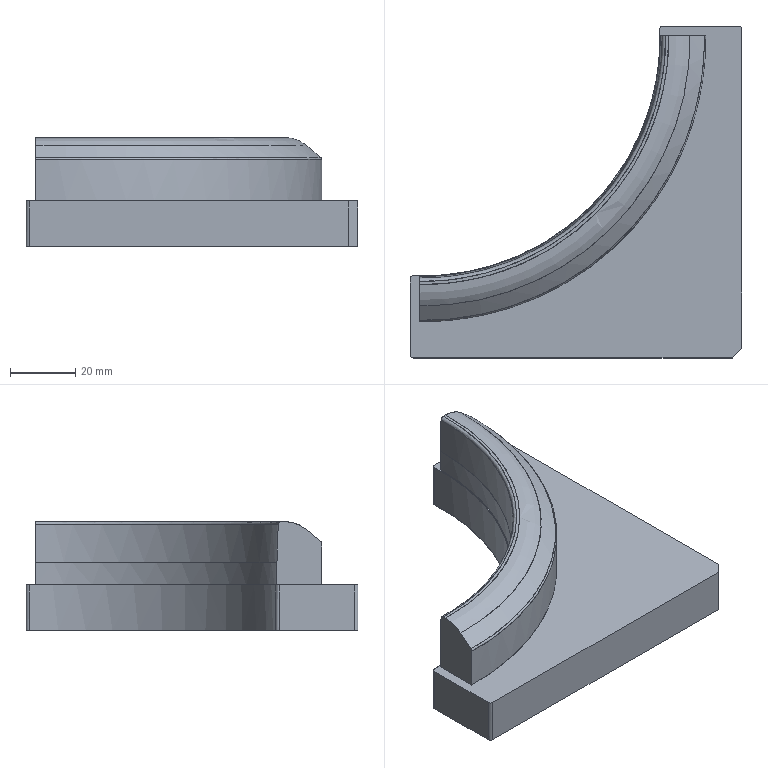NC program | PowerMill | posted with a generic post | part box 102 x 102 x 33.478 mm
Lines 27281 to 27988 of 205885:
N27378 M6
N27379 S18000 M03
N27380 G00 G90 X0.0 Y0.0
N27381 G43 Z10.798 H7
N27382
N27383 G05 P10000 R8
N27384 X16.2265 Y-15.1208
N27385 Z-7.8611
N27386 G01 Z-9.0611 F1200.0
N27387 X16.2193 Y-15.128 Z-9.0578 F2000.0
N27388 X16.1176 Y-15.2297 Z-9.0126
N27389 X16.0433 Y-15.304 Z-8.9841
N27390 X15.9799 Y-15.3673 Z-8.9661
N27391 X15.9402 Y-15.4071 Z-8.9595
N27392 X15.9003 Y-15.447 Z-8.9553
N27393 X15.8603 Y-15.4869 Z-8.9522
N27394 X15.7961 Y-15.5511 Z-8.9488
N27395 X15.7542 Y-15.593 Z-8.9473
N27396 X15.7142 Y-15.6331 Z-8.9464
N27397 X15.6741 Y-15.6732 Z-8.9466
N27398 X15.5794 Y-15.7678 Z-8.952
N27399 X15.4849 Y-15.8624 Z-8.9611
N27400 X15.39 Y-15.9572 Z-8.972
N27401 X15.2955 Y-16.0517 Z-8.9829
N27402 X15.2717 Y-16.0756 Z-8.9874
N27403 X15.2451 Y-16.1021 Z-8.9994
N27404 X15.2228 Y-16.1245 Z-9.0128
N27405 X15.1913 Y-16.1559 Z-9.0307
N27406 X15.1262 Y-16.2211 Z-9.0616
N27407 X13.2708 Y-17.9916 Z-9.0896
N27408 Z-9.0776
N27409 X13.2828 Y-17.9797 Z-9.0118
N27410 X13.2897 Y-17.9727 Z-8.9971
N27411 X13.3018 Y-17.9606 Z-8.9768
N27412 X13.3197 Y-17.9427 Z-8.9513
N27413 X13.3315 Y-17.931 Z-8.9371
N27414 X13.3421 Y-17.9203 Z-8.9277
N27415 X13.4059 Y-17.8566 Z-8.8821
N27416 X13.4779 Y-17.7845 Z-8.839
N27417 X13.5611 Y-17.7013 Z-8.7974
N27418 X13.6507 Y-17.6117 Z-8.7595
N27419 X13.7504 Y-17.512 Z-8.725
N27420 X13.8798 Y-17.3826 Z-8.687
N27421 X13.9702 Y-17.2922 Z-8.6636
N27422 X14.0609 Y-17.2015 Z-8.6432
N27423 X14.1517 Y-17.1107 Z-8.6243
N27424 X14.2427 Y-17.0197 Z-8.6067
N27425 X14.3339 Y-16.9286 Z-8.5905
N27426 X14.4252 Y-16.8372 Z-8.5767
N27427 X14.6885 Y-16.5739 Z-8.544
N27428 X14.9492 Y-16.3132 Z-8.5196
N27429 X15.2071 Y-16.0553 Z-8.5032
N27430 X15.4446 Y-15.8178 Z-8.4956
N27431 X15.7078 Y-15.5546 Z-8.4947
N27432 X15.9119 Y-15.3505 Z-8.4985
N27433 X16.1159 Y-15.1465 Z-8.5074
N27434 X16.3198 Y-14.9426 Z-8.5207
N27435 X16.5235 Y-14.7389 Z-8.5386
N27436 X16.7085 Y-14.5539 Z-8.5597
N27437 X16.8688 Y-14.3936 Z-8.5812
N27438 X17.0288 Y-14.2336 Z-8.6073
N27439 X17.1882 Y-14.0742 Z-8.6393
N27440 X17.2823 Y-13.9801 Z-8.6608
N27441 X17.4045 Y-13.8579 Z-8.6947
N27442 X17.4662 Y-13.7962 Z-8.7117
N27443 X17.506 Y-13.7564 Z-8.723
N27444 X17.5458 Y-13.7166 Z-8.7357
N27445 X17.5941 Y-13.6683 Z-8.7528
N27446 X17.6545 Y-13.6079 Z-8.7767
N27447 X17.7319 Y-13.5306 Z-8.812
N27448 X17.8001 Y-13.4623 Z-8.8488
N27449 X17.8538 Y-13.4086 Z-8.8833
N27450 X17.8968 Y-13.3656 Z-8.9163
N27451 X17.9314 Y-13.3311 Z-8.9484
N27452 X17.9522 Y-13.3102 Z-8.972
N27453 X17.9694 Y-13.293 Z-8.9998
N27454 X17.9824 Y-13.28 Z-9.0328
N27455 X17.9906 Y-13.2718 Z-9.0697
N27456 X17.9921 Y-13.2703 Z-9.0824
N27457 Z-9.0901
N27458 X18.8969 Y-12.2807 Z-9.0615
N27459 X18.8925 Y-12.285 Z-9.0442
N27460 X18.8789 Y-12.2987 Z-9.0058
N27461 X18.8582 Y-12.3194 Z-8.9636
N27462 X18.833 Y-12.3445 Z-8.9226
N27463 X18.8155 Y-12.3621 Z-8.8995
N27464 X18.7961 Y-12.3815 Z-8.8802
N27465 X18.7644 Y-12.4131 Z-8.8553
N27466 X18.7396 Y-12.438 Z-8.8355
N27467 X18.7035 Y-12.4741 Z-8.8076
N27468 X18.6614 Y-12.5162 Z-8.7799
N27469 X18.6104 Y-12.5671 Z-8.7504
N27470 X18.5454 Y-12.6322 Z-8.7168
N27471 X18.455 Y-12.7226 Z-8.6752
N27472 X18.3771 Y-12.8004 Z-8.6427
N27473 X18.3178 Y-12.8597 Z-8.6197
N27474 X18.2703 Y-12.9073 Z-8.6023
N27475 X18.2248 Y-12.9528 Z-8.5867
N27476 X18.1791 Y-12.9984 Z-8.5722
N27477 X18.103 Y-13.0746 Z-8.5503
N27478 X18.0267 Y-13.1509 Z-8.5296
N27479 X17.9503 Y-13.2273 Z-8.5095
N27480 X17.8697 Y-13.3078 Z-8.489
N27481 X17.7932 Y-13.3844 Z-8.4703
N27482 X17.7164 Y-13.4611 Z-8.4531
N27483 X17.6394 Y-13.5382 Z-8.4387
N27484 X17.4602 Y-13.7173 Z-8.4078
N27485 X17.2809 Y-13.8967 Z-8.3793
N27486 X17.1013 Y-14.0762 Z-8.3534
N27487 X16.9215 Y-14.256 Z-8.3317
N27488 X16.7123 Y-14.4653 Z-8.3122
N27489 X16.5029 Y-14.6746 Z-8.2962
N27490 X16.2935 Y-14.8841 Z-8.2832
N27491 X16.0839 Y-15.0936 Z-8.2736
N27492 X15.815 Y-15.3626 Z-8.2669
N27493 X15.4762 Y-15.7013 Z-8.2656
N27494 X15.1389 Y-16.0386 Z-8.2722
N27495 X14.936 Y-16.2416 Z-8.2803
N27496 X14.7331 Y-16.4445 Z-8.2919
N27497 X14.5303 Y-16.6473 Z-8.3068
N27498 X14.323 Y-16.8546 Z-8.3255
N27499 X14.1206 Y-17.057 Z-8.3479
N27500 X13.9185 Y-17.259 Z-8.3754
N27501 X13.7637 Y-17.4139 Z-8.4
N27502 X13.609 Y-17.5686 Z-8.4261
N27503 X13.4546 Y-17.723 Z-8.4556
N27504 X13.3008 Y-17.8768 Z-8.49
N27505 X13.1476 Y-18.0299 Z-8.53
N27506 X13.0554 Y-18.1221 Z-8.5567
N27507 X12.9635 Y-18.2141 Z-8.5851
N27508 X12.8718 Y-18.3057 Z-8.6155
N27509 X12.7807 Y-18.3968 Z-8.6487
N27510 X12.6905 Y-18.4871 Z-8.6862
N27511 X12.6162 Y-18.5613 Z-8.7234
N27512 X12.5356 Y-18.6419 Z-8.7718
N27513 X12.4413 Y-18.7362 Z-8.8361
N27514 X12.4063 Y-18.7713 Z-8.8615
N27515 X12.3731 Y-18.8044 Z-8.8915
N27516 X12.3433 Y-18.8342 Z-8.9278
N27517 X12.3174 Y-18.8602 Z-8.9699
N27518 X12.296 Y-18.8816 Z-9.0168
N27519 X12.2794 Y-18.8981 Z-9.0676
N27520 X11.518 Y-19.5747 Z-9.1132
N27521 Z-9.0836
N27522 X11.5206 Y-19.5721 Z-9.0598
N27523 X11.5261 Y-19.5666 Z-9.0337
N27524 X11.5372 Y-19.5555 Z-8.9982
N27525 X11.5536 Y-19.5391 Z-8.957
N27526 X11.5659 Y-19.5268 Z-8.9309
N27527 X11.5748 Y-19.5179 Z-8.9148
N27528 X11.5787 Y-19.514 Z-8.909
N27529 X11.6088 Y-19.4839 Z-8.8732
N27530 X11.6397 Y-19.453 Z-8.839
N27531 X11.6717 Y-19.421 Z-8.8073
N27532 X11.7052 Y-19.3875 Z-8.7786
N27533 X11.7477 Y-19.345 Z-8.7486
N27534 X11.784 Y-19.3087 Z-8.7262
N27535 X11.8206 Y-19.2721 Z-8.7046
N27536 X11.8571 Y-19.2356 Z-8.6828
N27537 X11.8933 Y-19.1994 Z-8.6604
N27538 X11.9298 Y-19.1629 Z-8.6399
N27539 X11.969 Y-19.1237 Z-8.6209
N27540 X12.0116 Y-19.0811 Z-8.6019
N27541 X12.0651 Y-19.0276 Z-8.5796
N27542 X12.1346 Y-18.9581 Z-8.5523
N27543 X12.2414 Y-18.8513 Z-8.5129
N27544 X12.3127 Y-18.78 Z-8.4879
N27545 X12.3676 Y-18.7251 Z-8.4695
N27546 X12.4116 Y-18.6811 Z-8.4552
N27547 X12.4522 Y-18.6405 Z-8.4426
N27548 X12.493 Y-18.5997 Z-8.4309
N27549 X12.6543 Y-18.4384 Z-8.3875
N27550 X12.816 Y-18.2767 Z-8.3473
N27551 X12.9784 Y-18.1143 Z-8.3128
N27552 X13.2181 Y-17.8746 Z-8.269
N27553 X13.5054 Y-17.5874 Z-8.2236
N27554 X13.738 Y-17.3547 Z-8.1922
N27555 X13.9711 Y-17.1217 Z-8.1664
N27556 X14.211 Y-16.8817 Z-8.1443
N27557 X14.4444 Y-16.6483 Z-8.1265
N27558 X14.678 Y-16.4147 Z-8.1123
N27559 X14.9116 Y-16.1811 Z-8.1017
N27560 X15.2722 Y-15.8205 Z-8.0917
N27561 X15.6329 Y-15.4598 Z-8.0897
N27562 X15.9569 Y-15.1358 Z-8.0946
N27563 X16.2808 Y-14.8119 Z-8.106
N27564 X16.6045 Y-14.4882 Z-8.1236
N27565 X16.928 Y-14.1647 Z-8.1479
N27566 X17.1899 Y-13.9028 Z-8.1731
N27567 X17.4514 Y-13.6413 Z-8.2043
N27568 X17.7125 Y-13.3802 Z-8.2424
N27569 X17.9731 Y-13.1196 Z-8.2864
N27570 X18.1574 Y-12.9353 Z-8.3214
N27571 X18.3526 Y-12.7401 Z-8.3658
N27572 X18.5738 Y-12.5189 Z-8.4236
N27573 X18.7134 Y-12.3793 Z-8.4638
N27574 X18.856 Y-12.2367 Z-8.512
N27575 X19.0069 Y-12.0858 Z-8.571
N27576 X19.0478 Y-12.0449 Z-8.5883
N27577 X19.1472 Y-11.9455 Z-8.634
N27578 X19.228 Y-11.8647 Z-8.6764
N27579 X19.295 Y-11.7978 Z-8.7162
N27580 X19.3511 Y-11.7416 Z-8.754
N27581 X19.3983 Y-11.6944 Z-8.7902
N27582 X19.4374 Y-11.6553 Z-8.825
N27583 X19.4707 Y-11.622 Z-8.8601
N27584 X19.4891 Y-11.6036 Z-8.8828
N27585 X19.5052 Y-11.5875 Z-8.9024
N27586 X19.5213 Y-11.5715 Z-8.9219
N27587 X19.5371 Y-11.5556 Z-8.9453
N27588 X19.5485 Y-11.5442 Z-8.9686
N27589 X19.558 Y-11.5347 Z-8.9937
N27590 X19.5651 Y-11.5276 Z-9.0157
N27591 X19.5699 Y-11.5228 Z-9.0391
N27592 X19.5739 Y-11.5188 Z-9.074
N27593 X19.5743 Y-11.5184 Z-9.0765
N27594 Z-9.1072
N27595 X20.1413 Y-10.8666 Z-9.0633
N27596 X20.1412 Y-10.8667 Z-9.0626
N27597 X20.1332 Y-10.8746 Z-9.0132
N27598 X20.1247 Y-10.8832 Z-8.9792
N27599 X20.114 Y-10.8938 Z-8.9541
N27600 X20.0833 Y-10.9246 Z-8.9013
N27601 X20.0491 Y-10.9587 Z-8.8526
N27602 X20.0109 Y-10.997 Z-8.8076
N27603 X19.9674 Y-11.0405 Z-8.7654
N27604 X19.9163 Y-11.0915 Z-8.7246
N27605 X19.8522 Y-11.1557 Z-8.6811
N27606 X19.7587 Y-11.2491 Z-8.6234
N27607 X19.6608 Y-11.3471 Z-8.5699
N27608 X19.5517 Y-11.4562 Z-8.5183
N27609 X19.4263 Y-11.5816 Z-8.467
N27610 X19.2723 Y-11.7355 Z-8.4112
N27611 X19.1728 Y-11.8351 Z-8.3774
N27612 X19.0434 Y-11.9644 Z-8.338
N27613 X18.9135 Y-12.0943 Z-8.3027
N27614 X18.7539 Y-12.2539 Z-8.263
N27615 X18.6233 Y-12.3846 Z-8.2328
N27616 X18.4925 Y-12.5154 Z-8.2042
N27617 X18.3542 Y-12.6536 Z-8.1768
N27618 X18.1829 Y-12.8249 Z-8.1467
N27619 X18.0113 Y-12.9965 Z-8.1194
N27620 X17.8396 Y-13.1683 Z-8.0942
N27621 X17.6677 Y-13.3402 Z-8.0709
N27622 X17.3611 Y-13.6467 Z-8.0352
N27623 X17.0339 Y-13.974 Z-8.0048
N27624 X16.6801 Y-14.3277 Z-7.9797
N27625 X16.2895 Y-14.7184 Z-7.9595
N27626 X16.1584 Y-14.8495 Z-7.9549
N27627 X16.0272 Y-14.9807 Z-7.9512
N27628 X15.896 Y-15.1118 Z-7.9479
N27629 X15.7649 Y-15.243 Z-7.9452
N27630 X15.4503 Y-15.5576 Z-7.9437
N27631 X15.0558 Y-15.9521 Z-7.9489
N27632 X14.6623 Y-16.3456 Z-7.9622
N27633 X14.2698 Y-16.738 Z-7.9833
N27634 X14.0453 Y-16.9625 Z-7.999
N27635 X13.821 Y-17.1869 Z-8.0181
N27636 X13.5967 Y-17.4111 Z-8.0406
N27637 X13.3727 Y-17.6351 Z-8.0664
N27638 X13.149 Y-17.8589 Z-8.0967
N27639 X12.8773 Y-18.1305 Z-8.1382
N27640 X12.6499 Y-18.358 Z-8.1774
N27641 X12.5531 Y-18.4547 Z-8.1965
N27642 X12.4565 Y-18.5514 Z-8.217
N27643 X12.36 Y-18.6479 Z-8.2384
N27644 X12.2635 Y-18.7443 Z-8.2606
N27645 X12.1672 Y-18.8406 Z-8.2837
N27646 X12.0711 Y-18.9368 Z-8.3081
N27647 X11.9752 Y-19.0326 Z-8.3346
N27648 X11.8798 Y-19.1281 Z-8.3644
N27649 X11.7783 Y-19.2296 Z-8.3969
N27650 X11.6769 Y-19.3309 Z-8.4306
N27651 X11.5668 Y-19.4411 Z-8.4709
N27652 X11.467 Y-19.5408 Z-8.5122
N27653 X11.3684 Y-19.6395 Z-8.5583
N27654 X11.2708 Y-19.737 Z-8.6089
N27655 X11.2003 Y-19.8076 Z-8.6489
N27656 X11.1276 Y-19.8803 Z-8.6962
N27657 X11.0661 Y-19.9418 Z-8.7432
N27658 X11.014 Y-19.9938 Z-8.7906
N27659 X10.9752 Y-20.0327 Z-8.8327
N27660 X10.937 Y-20.0708 Z-8.8832
N27661 X10.8932 Y-20.1146 Z-8.9506
N27662 X10.8824 Y-20.1255 Z-8.982
N27663 X10.871 Y-20.1369 Z-9.0303
N27664 X10.865 Y-20.1428 Z-9.0806
N27665 Z-9.0816
N27666 X10.2807 Y-20.6423 Z-9.0991
N27667 Z-9.0832
N27668 X10.2841 Y-20.6389 Z-9.043
N27669 X10.2908 Y-20.6322 Z-9.0038
N27670 X10.3022 Y-20.6208 Z-8.9661
N27671 X10.3174 Y-20.6056 Z-8.9318
N27672 X10.3352 Y-20.5878 Z-8.8991
N27673 X10.3678 Y-20.5552 Z-8.849
N27674 X10.407 Y-20.516 Z-8.8002
N27675 X10.4538 Y-20.4692 Z-8.7522
N27676 X10.5094 Y-20.4136 Z-8.7042
N27677 X10.5762 Y-20.3468 Z-8.6551
N27678 X10.6291 Y-20.2939 Z-8.6202
N27679 X10.7281 Y-20.1949 Z-8.5604
N27680 X10.8287 Y-20.0943 Z-8.5061
N27681 X10.9308 Y-19.9922 Z-8.4575
N27682 X11.0391 Y-19.8839 Z-8.412
N27683 X11.1433 Y-19.7797 Z-8.3725
N27684 X11.2478 Y-19.6752 Z-8.3353
N27685 X11.4165 Y-19.5065 Z-8.2809
N27686 X11.6143 Y-19.3087 Z-8.2247
N27687 X11.8201 Y-19.1029 Z-8.1719
N27688 X12.0406 Y-18.8824 Z-8.1225
N27689 X12.3038 Y-18.6192 Z-8.0707
N27690 X12.5005 Y-18.4225 Z-8.0354
N27691 X12.6977 Y-18.2253 Z-8.0047
N27692 X12.895 Y-18.028 Z-7.9773
N27693 X13.0925 Y-17.8305 Z-7.9518
N27694 X13.2902 Y-17.6328 Z-7.9283
N27695 X13.5397 Y-17.3833 Z-7.9032
N27696 X13.7895 Y-17.1335 Z-7.8815
N27697 X14.0394 Y-16.8836 Z-7.8632
N27698 X14.2894 Y-16.6336 Z-7.8486
N27699 X14.6538 Y-16.2692 Z-7.8326
N27700 X15.0183 Y-15.9047 Z-7.822
N27701 X15.3829 Y-15.5401 Z-7.8174
N27702 X15.7601 Y-15.1629 Z-7.8196
N27703 X16.1372 Y-14.7858 Z-7.8281
N27704 X16.5143 Y-14.4087 Z-7.8426
N27705 X16.8689 Y-14.0541 Z-7.8623
N27706 X17.2233 Y-13.6997 Z-7.8888
N27707 X17.5774 Y-13.3456 Z-7.9228
N27708 X17.9311 Y-12.9919 Z-7.9643
N27709 X18.1871 Y-12.7359 Z-7.9987
N27710 X18.4426 Y-12.4804 Z-8.039
N27711 X18.6976 Y-12.2254 Z-8.0855
N27712 X18.952 Y-11.971 Z-8.1378
N27713 X19.0809 Y-11.8421 Z-8.1666
N27714 X19.2094 Y-11.7136 Z-8.1981
N27715 X19.3376 Y-11.5854 Z-8.2322
N27716 X19.4822 Y-11.4408 Z-8.2739
N27717 X19.6095 Y-11.3135 Z-8.3135
N27718 X19.7363 Y-11.1867 Z-8.3565
N27719 X19.8623 Y-11.0607 Z-8.4042
N27720 X19.969 Y-10.954 Z-8.4488
N27721 X20.0876 Y-10.8354 Z-8.5035
N27722 X20.1634 Y-10.7596 Z-8.5427
N27723 X20.2476 Y-10.6754 Z-8.5903
N27724 X20.3319 Y-10.5911 Z-8.6437
N27725 X20.4041 Y-10.5189 Z-8.6966
N27726 X20.4709 Y-10.4521 Z-8.7535
N27727 X20.4973 Y-10.4257 Z-8.7785
N27728 X20.5195 Y-10.4035 Z-8.8028
N27729 X20.5441 Y-10.3789 Z-8.8347
N27730 X20.5757 Y-10.3473 Z-8.8825
N27731 X20.5998 Y-10.3232 Z-8.9256
N27732 X20.6156 Y-10.3074 Z-8.9603
N27733 X20.6262 Y-10.2968 Z-8.9908
N27734 X20.6368 Y-10.2862 Z-9.0304
N27735 X20.6415 Y-10.2815 Z-9.0635
N27736 X20.642 Y-10.281 Z-9.0766
N27737 Z-9.1018
N27738 X21.0919 Y-9.7462 Z-9.1082
N27739 Z-9.0725
N27740 Z-9.0709
N27741 X21.0896 Y-9.7486 Z-9.0535
N27742 X21.0871 Y-9.751 Z-9.0393
N27743 X21.0835 Y-9.7547 Z-9.0214
N27744 X21.0764 Y-9.7617 Z-8.993
N27745 X21.0663 Y-9.7718 Z-8.9581
N27746 X21.0592 Y-9.779 Z-8.9373
N27747 X21.0537 Y-9.7845 Z-8.9251
N27748 X21.0314 Y-9.8067 Z-8.8882
N27749 X21.0007 Y-9.8375 Z-8.8401
N27750 X20.9678 Y-9.8703 Z-8.795
N27751 X20.9324 Y-9.9057 Z-8.7541
N27752 X20.8947 Y-9.9434 Z-8.7175
N27753 X20.8556 Y-9.9826 Z-8.684
N27754 X20.8156 Y-10.0225 Z-8.6524
N27755 X20.7753 Y-10.0628 Z-8.622
N27756 X20.6917 Y-10.1464 Z-8.5649
N27757 X20.5988 Y-10.2394 Z-8.5099
N27758 X20.4936 Y-10.3445 Z-8.4558
N27759 X20.3904 Y-10.4477 Z-8.4075
N27760 X20.2744 Y-10.5638 Z-8.3567
N27761 X20.1573 Y-10.6808 Z-8.3107
N27762 X20.0393 Y-10.7988 Z-8.2694
N27763 X19.9208 Y-10.9173 Z-8.2312
N27764 X19.8021 Y-11.036 Z-8.1941
N27765 X19.6844 Y-11.1537 Z-8.1598
N27766 X19.5663 Y-11.2718 Z-8.1285
N27767 X19.448 Y-11.3901 Z-8.0989
N27768 X19.3295 Y-11.5086 Z-8.0707
N27769 X19.2109 Y-11.6273 Z-8.0438
N27770 X19.092 Y-11.7461 Z-8.0191
N27771 X18.8211 Y-12.0171 Z-7.9689
N27772 X18.5074 Y-12.3308 Z-7.9167
N27773 X18.2154 Y-12.6227 Z-7.8752
N27774 X17.8486 Y-12.9896 Z-7.8311
N27775 X17.4813 Y-13.3569 Z-7.794
N27776 X17.1137 Y-13.7245 Z-7.7639
N27777 X16.7246 Y-14.1135 Z-7.7393
N27778 X16.3354 Y-14.5027 Z-7.722
N27779 X15.9669 Y-14.8713 Z-7.7113
N27780 X15.5983 Y-15.2399 Z-7.7058
N27781 X15.2297 Y-15.6085 Z-7.7061
N27782 X14.7843 Y-16.0539 Z-7.7132
N27783 X14.3441 Y-16.494 Z-7.7281
N27784 X14.0453 Y-16.7928 Z-7.7433
N27785 X13.7466 Y-17.0915 Z-7.7625
N27786 X13.448 Y-17.3901 Z-7.7856
N27787 X13.2149 Y-17.6233 Z-7.8076
N27788 X12.9818 Y-17.8563 Z-7.8323
N27789 X12.7489 Y-18.0893 Z-7.8593
N27790 X12.5161 Y-18.322 Z-7.889
N27791 X12.3818 Y-18.4564 Z-7.9081
N27792 X12.2476 Y-18.5906 Z-7.9295
N27793 X12.1135 Y-18.7247 Z-7.9522
N27794 X11.9794 Y-18.8587 Z-7.9758
N27795 X11.8455 Y-18.9926 Z-8.0005
N27796 X11.7117 Y-19.1264 Z-8.0265
N27797 X11.5782 Y-19.2599 Z-8.055
N27798 X11.335 Y-19.5032 Z-8.1129
N27799 X11.1248 Y-19.7134 Z-8.168
N27800 X11.0262 Y-19.812 Z-8.1964
N27801 X10.9278 Y-19.9103 Z-8.2266
N27802 X10.8251 Y-20.013 Z-8.2603
N27803 X10.6985 Y-20.1397 Z-8.3051
N27804 X10.5457 Y-20.2925 Z-8.3645
N27805 X10.4274 Y-20.4107 Z-8.4157
N27806 X10.3305 Y-20.5076 Z-8.462
N27807 X10.2365 Y-20.6016 Z-8.512
N27808 X10.1667 Y-20.6714 Z-8.5536
N27809 X10.077 Y-20.7611 Z-8.6115
N27810 X10.0069 Y-20.8312 Z-8.6628
N27811 X9.9482 Y-20.89 Z-8.7131
N27812 X9.8976 Y-20.9405 Z-8.7643
N27813 X9.8535 Y-20.9847 Z-8.8178
N27814 X9.8304 Y-21.0078 Z-8.8495
N27815 X9.8091 Y-21.029 Z-8.8809
N27816 X9.7896 Y-21.0485 Z-8.9146
N27817 X9.7734 Y-21.0648 Z-8.9519
N27818 X9.7615 Y-21.0767 Z-8.9917
N27819 X9.7528 Y-21.0853 Z-9.0333
N27820 X9.746 Y-21.0922 Z-9.0756
N27821 Z-9.1074
N27822 X9.2611 Y-21.4922 Z-9.061
N27823 X9.2649 Y-21.4884 Z-9.0207
N27824 X9.2732 Y-21.4801 Z-8.9806
N27825 X9.2874 Y-21.4659 Z-8.9381
N27826 X9.3045 Y-21.4488 Z-8.8988
N27827 X9.3308 Y-21.4225 Z-8.8498
N27828 X9.3634 Y-21.3899 Z-8.8014
N27829 X9.4036 Y-21.3497 Z-8.7527
N27830 X9.4535 Y-21.2998 Z-8.7019
N27831 X9.5071 Y-21.2462 Z-8.654
N27832 X9.579 Y-21.1743 Z-8.5966
N27833 X9.6604 Y-21.0929 Z-8.5403
N27834 X9.7554 Y-20.9979 Z-8.483
N27835 X9.8729 Y-20.8804 Z-8.4196
N27836 X9.9927 Y-20.7606 Z-8.3616
N27837 X10.1299 Y-20.6234 Z-8.303
N27838 X10.2978 Y-20.4555 Z-8.2387
N27839 X10.4 Y-20.3533 Z-8.2018
N27840 X10.5028 Y-20.2505 Z-8.1685
N27841 X10.6059 Y-20.1474 Z-8.1373
N27842 X10.7092 Y-20.044 Z-8.1074
N27843 X10.8127 Y-19.9406 Z-8.0786
N27844 X10.9164 Y-19.8369 Z-8.0508
N27845 X11.0202 Y-19.7331 Z-8.0246
N27846 X11.1243 Y-19.629 Z-8.0007
N27847 X11.3783 Y-19.375 Z-7.946
N27848 X11.6328 Y-19.1204 Z-7.8966
N27849 X11.888 Y-18.8653 Z-7.8534
N27850 X12.1434 Y-18.6099 Z-7.8145
N27851 X12.3991 Y-18.3542 Z-7.779
N27852 X12.7088 Y-18.0445 Z-7.742
N27853 X13.0432 Y-17.7101 Z-7.7081
N27854 X13.3534 Y-17.3999 Z-7.6814
N27855 X13.6638 Y-17.0895 Z-7.6585
N27856 X14.077 Y-16.6763 Z-7.6344
N27857 X14.5028 Y-16.2505 Z-7.6171
N27858 X14.9549 Y-15.7984 Z-7.6066
N27859 X15.3833 Y-15.37 Z-7.6035
N27860 X15.8491 Y-14.9042 Z-7.6074
N27861 X16.3032 Y-14.4501 Z-7.6189
N27862 X16.7467 Y-14.0066 Z-7.6379
N27863 X17.1576 Y-13.5957 Z-7.663
N27864 X17.5842 Y-13.1691 Z-7.6969
N27865 X17.9183 Y-12.835 Z-7.7287
N27866 X18.252 Y-12.5013 Z-7.7661
N27867 X18.5853 Y-12.1679 Z-7.8106
N27868 X18.8431 Y-11.9102 Z-7.8498
N27869 X19.1006 Y-11.6527 Z-7.893
N27870 X19.3575 Y-11.3958 Z-7.9424
N27871 X19.5574 Y-11.1958 Z-7.9842
N27872 X19.7971 Y-10.9562 Z-8.04
N27873 X20.0184 Y-10.7349 Z-8.0988
N27874 X20.2254 Y-10.5279 Z-8.1612
N27875 X20.3961 Y-10.3572 Z-8.2187
N27876 X20.5023 Y-10.251 Z-8.2565
N27877 X20.6083 Y-10.145 Z-8.2957
N27878 X20.7134 Y-10.0399 Z-8.3389
N27879 X20.817 Y-9.9362 Z-8.3884
N27880 X20.9197 Y-9.8336 Z-8.4421
N27881 X20.9901 Y-9.7632 Z-8.4804
N27882 X21.0514 Y-9.7019 Z-8.5147
N27883 X21.1121 Y-9.6412 Z-8.5512
N27884 X21.1715 Y-9.5818 Z-8.5913
N27885 X21.2291 Y-9.5242 Z-8.6364
N27886 X21.2845 Y-9.4688 Z-8.6865
N27887 X21.338 Y-9.4153 Z-8.7407
N27888 X21.3672 Y-9.3861 Z-8.7721
N27889 X21.3799 Y-9.3734 Z-8.788
N27890 X21.3953 Y-9.358 Z-8.8097
N27891 X21.4191 Y-9.3342 Z-8.8459
N27892 X21.4356 Y-9.3177 Z-8.873
N27893 X21.4461 Y-9.3071 Z-8.8918
N27894 X21.4554 Y-9.2979 Z-8.9119
N27895 X21.4737 Y-9.2796 Z-8.9605
N27896 X21.4855 Y-9.2678 Z-9.0038
N27897 X21.4913 Y-9.262 Z-9.0423
N27898 X21.4922 Y-9.2611 Z-9.0632
N27899 X21.8673 Y-8.8012 Z-9.1297
N27900 Z-9.072
N27901 X21.8671 Y-8.8013 Z-9.0699
N27902 X21.8633 Y-8.8051 Z-9.016
N27903 X21.8572 Y-8.8112 Z-8.977
N27904 X21.8475 Y-8.8209 Z-8.9446
N27905 X21.8393 Y-8.8291 Z-8.9257
N27906 X21.8282 Y-8.8402 Z-8.9025
N27907 X21.8105 Y-8.858 Z-8.8674
N27908 X21.7911 Y-8.8773 Z-8.8318
N27909 X21.7778 Y-8.8907 Z-8.8095
N27910 X21.7667 Y-8.9017 Z-8.794
N27911 X21.7528 Y-8.9156 Z-8.778
N27912 X21.7027 Y-8.9657 Z-8.721
N27913 X21.6515 Y-9.017 Z-8.666
N27914 X21.5978 Y-9.0707 Z-8.6161
N27915 X21.5415 Y-9.127 Z-8.5725
N27916 X21.4836 Y-9.1848 Z-8.533
N27917 X21.4251 Y-9.2433 Z-8.4955
N27918 X21.3662 Y-9.3022 Z-8.4593
N27919 X21.247 Y-9.4214 Z-8.3919
N27920 X21.1183 Y-9.5501 Z-8.3275
N27921 X20.9777 Y-9.6907 Z-8.2653
N27922 X20.8211 Y-9.8473 Z-8.204
N27923 X20.6405 Y-10.028 Z-8.1408
N27924 X20.4152 Y-10.2532 Z-8.0693
N27925 X20.2912 Y-10.3772 Z-8.0329
N27926 X20.1362 Y-10.5322 Z-7.9924
N27927 X19.969 Y-10.6994 Z-7.9518
N27928 X19.8136 Y-10.8549 Z-7.9149
N27929 X19.6266 Y-11.0418 Z-7.8754
N27930 X19.4393 Y-11.2292 Z-7.8395
N27931 X19.2518 Y-11.4167 Z-7.8055
N27932 X18.947 Y-11.7215 Z-7.7553
N27933 X18.6416 Y-12.0268 Z-7.7122
N27934 X18.29 Y-12.3784 Z-7.6684
N27935 X17.9381 Y-12.7304 Z-7.6307
N27936 X17.5858 Y-13.0827 Z-7.5995
N27937 X17.2333 Y-13.4352 Z-7.5735
N27938 X16.7928 Y-13.8756 Z-7.5474
N27939 X16.3521 Y-14.3163 Z-7.5284
N27940 X15.8791 Y-14.7894 Z-7.5157
N27941 X15.3988 Y-15.2696 Z-7.5107
N27942 X14.9442 Y-15.7242 Z-7.5132
N27943 X14.4896 Y-16.1788 Z-7.5227
N27944 X14.0352 Y-16.6333 Z-7.5397
N27945 X13.5809 Y-17.0876 Z-7.5643
N27946 X13.196 Y-17.4725 Z-7.5904
N27947 X12.8349 Y-17.8336 Z-7.6207
N27948 X12.4741 Y-18.1943 Z-7.6577
N27949 X12.191 Y-18.4774 Z-7.6913
N27950 X11.9081 Y-18.7603 Z-7.7281
N27951 X11.7419 Y-18.9266 Z-7.7517
N27952 X11.5759 Y-19.0926 Z-7.7782
N27953 X11.41 Y-19.2584 Z-7.8068
N27954 X11.2443 Y-19.4242 Z-7.8368
N27955 X11.0787 Y-19.5898 Z-7.8682
N27956 X10.9133 Y-19.7551 Z-7.9019
N27957 X10.7483 Y-19.9201 Z-7.9394
N27958 X10.5566 Y-20.1119 Z-7.9866
N27959 X10.3653 Y-20.3032 Z-8.0373
N27960 X10.1746 Y-20.4938 Z-8.0926
N27961 X10.0934 Y-20.575 Z-8.1181
N27962 X10.0124 Y-20.6561 Z-8.1451
N27963 X9.925 Y-20.7434 Z-8.1758
N27964 X9.8204 Y-20.848 Z-8.2147
N27965 X9.6891 Y-20.9793 Z-8.2673
N27966 X9.5499 Y-21.1186 Z-8.3285
N27967 X9.4412 Y-21.2272 Z-8.381
N27968 X9.3517 Y-21.3168 Z-8.4286
N27969 X9.2751 Y-21.3934 Z-8.4733
N27970 X9.1998 Y-21.4687 Z-8.5223
N27971 X9.1443 Y-21.5242 Z-8.5628
N27972 X9.0662 Y-21.6022 Z-8.6228
N27973 X9.0088 Y-21.6596 Z-8.6725
N27974 X8.9623 Y-21.7061 Z-8.72
N27975 X8.9236 Y-21.7449 Z-8.768
N27976 X8.9019 Y-21.7665 Z-8.7981
N27977 X8.8784 Y-21.7901 Z-8.8322
N27978 X8.8572 Y-21.8113 Z-8.8661
N27979 X8.8386 Y-21.8299 Z-8.9019
N27980 X8.8231 Y-21.8453 Z-8.9425
N27981 X8.8128 Y-21.8556 Z-8.984
N27982 X8.806 Y-21.8624 Z-9.0268
N27983 X8.8012 Y-21.8672 Z-9.072
N27984 Y-21.8673 Z-9.1088
N27985 X8.3592 Y-22.2244 Z-9.0964
N27986 Z-9.0834
N27987 X8.3642 Y-22.2194 Z-9.0312
N27988 X8.3749 Y-22.2087 Z-8.9772
N27989 X8.3896 Y-22.194 Z-8.9296
N27990 X8.412 Y-22.1715 Z-8.8771
N27991 X8.4411 Y-22.1425 Z-8.8241
N27992 X8.4773 Y-22.1062 Z-8.7702
N27993 X8.5217 Y-22.0618 Z-8.7152
N27994 X8.5743 Y-22.0093 Z-8.6596
N27995 X8.6308 Y-21.9528 Z-8.6073
N27996 X8.7037 Y-21.8799 Z-8.5485
N27997 X8.7876 Y-21.796 Z-8.4895
N27998 X8.8878 Y-21.6958 Z-8.4271
N27999 X9.0151 Y-21.5685 Z-8.3555
N28000 X9.1492 Y-21.4343 Z-8.2883
N28001 X9.2951 Y-21.2884 Z-8.2233
N28002 X9.427 Y-21.1566 Z-8.1706
N28003 X9.5932 Y-20.9904 Z-8.1092
N28004 X9.7604 Y-20.8232 Z-8.0537
N28005 X9.9285 Y-20.6551 Z-8.0041
N28006 X10.1336 Y-20.45 Z-7.9471
N28007 X10.3392 Y-20.2444 Z-7.8945
N28008 X10.5456 Y-20.038 Z-7.848
N28009 X10.7523 Y-19.8313 Z-7.8046
N28010 X11.0157 Y-19.5679 Z-7.7541
N28011 X11.2888 Y-19.2948 Z-7.7083
N28012 X11.553 Y-19.0306 Z-7.6678
N28013 X11.8748 Y-18.7087 Z-7.6234
N28014 X12.1971 Y-18.3865 Z-7.5853
N28015 X12.5196 Y-18.064 Z-7.5521
N28016 X12.8423 Y-17.7413 Z-7.5229
N28017 X13.1651 Y-17.4184 Z-7.4978
N28018 X13.5764 Y-17.0072 Z-7.4721
N28019 X14.0541 Y-16.5295 Z-7.4498
N28020 X14.5319 Y-16.0517 Z-7.4349
N28021 X15.0098 Y-15.5738 Z-7.4271
N28022 X15.4544 Y-15.1291 Z-7.4262
N28023 X15.8991 Y-14.6845 Z-7.4316
N28024 X16.3437 Y-14.2399 Z-7.4432
N28025 X16.7882 Y-13.7954 Z-7.461
N28026 X17.2325 Y-13.3511 Z-7.4854
N28027 X17.5483 Y-13.0353 Z-7.5072
N28028 X17.8639 Y-12.7197 Z-7.5333
N28029 X18.3129 Y-12.2707 Z-7.5775
N28030 X18.6426 Y-11.941 Z-7.6151
N28031 X18.981 Y-11.6026 Z-7.6604
N28032 X19.333 Y-11.2506 Z-7.7142
N28033 X19.6299 Y-10.9537 Z-7.7655
N28034 X19.9085 Y-10.6751 Z-7.8205
N28035 X20.1804 Y-10.4031 Z-7.8802
N28036 X20.4202 Y-10.1634 Z-7.9395
N28037 X20.6156 Y-9.968 Z-7.9931
N28038 X20.8104 Y-9.7732 Z-8.051
N28039 X21.0042 Y-9.5794 Z-8.1149
N28040 X21.1805 Y-9.4031 Z-8.1785
N28041 X21.2285 Y-9.355 Z-8.1977
N28042 X21.2764 Y-9.3072 Z-8.2182
N28043 X21.3253 Y-9.2583 Z-8.2399
N28044 X21.3902 Y-9.1934 Z-8.2696
N28045 X21.48 Y-9.1036 Z-8.3118
N28046 X21.5392 Y-9.0444 Z-8.3404
N28047 X21.5863 Y-8.9973 Z-8.3639
N28048 X21.6332 Y-8.9504 Z-8.3882
N28049 X21.6758 Y-8.9078 Z-8.412
N28050 X21.7127 Y-8.8709 Z-8.435
N28051 X21.7579 Y-8.8257 Z-8.4646
N28052 X21.8169 Y-8.7667 Z-8.5053
N28053 X21.8967 Y-8.6869 Z-8.5641
N28054 X21.9508 Y-8.6328 Z-8.6075
N28055 X21.9919 Y-8.5917 Z-8.6433
N28056 X22.025 Y-8.5585 Z-8.6752
N28057 X22.0565 Y-8.5271 Z-8.7106
N28058 X22.1065 Y-8.477 Z-8.7741
N28059 X22.143 Y-8.4406 Z-8.8275
N28060 X22.1711 Y-8.4125 Z-8.8778
N28061 X22.1927 Y-8.3909 Z-8.9274
N28062 X22.2072 Y-8.3763 Z-8.9724
N28063 X22.2167 Y-8.3669 Z-9.0164
N28064 X22.2239 Y-8.3597 Z-9.0734
N28065 X22.2241 Y-8.3595 Z-9.0754
N28066 Z-9.0943
N28067 X22.5486 Y-7.9501 Z-9.0764
N28068 Z-9.0696
N28069 X22.5456 Y-7.9532 Z-9.0422
N28070 X22.5355 Y-7.9632 Z-8.9804
N28071 X22.5221 Y-7.9766 Z-8.9275
N28072 X22.5083 Y-7.9904 Z-8.8894
N28073 X22.4911 Y-8.0076 Z-8.854
N28074 X22.4652 Y-8.0336 Z-8.8066
N28075 X22.4341 Y-8.0646 Z-8.7599
N28076 X22.3935 Y-8.1052 Z-8.7093
N28077 X22.3397 Y-8.159 Z-8.651
N28078 X22.2795 Y-8.2193 Z-8.5935
N28079 X22.2117 Y-8.287 Z-8.5368
N28080 X22.1323 Y-8.3664 Z-8.4782
N28081 X22.0382 Y-8.4605 Z-8.4164
N28082 X21.9261 Y-8.5727 Z-8.3509
N28083 X21.8199 Y-8.6788 Z-8.2949
N28084 X21.7311 Y-8.7676 Z-8.2514
N28085 X21.653 Y-8.8457 Z-8.2154